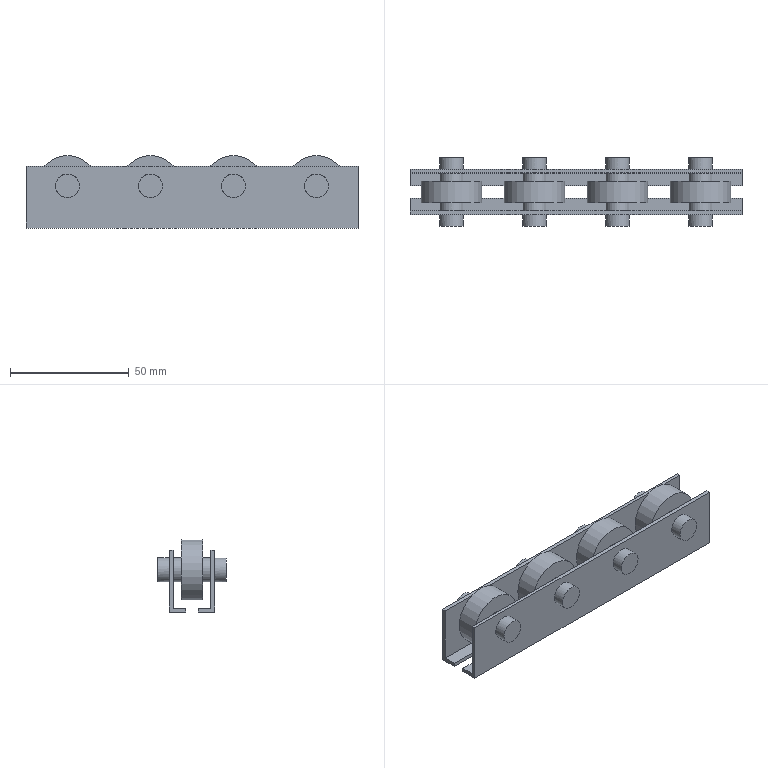Part | NX | features solid 2 | 1 solid | 52 faces | box 140 x 29 x 30.5 mm | volume 37587 mm3 | plane 32 | cylinder 20 | commonest cylinder face diameters 10 x16 25.4 x4
STEP:
#1=CARTESIAN_POINT('',(-1407.5,158.,-11.7));
#2=VERTEX_POINT('',#1);
#3=CARTESIAN_POINT('',(-1407.5,158.,-16.7));
#4=DIRECTION('',(0.,1.,0.));
#5=DIRECTION('',(0.,0.,1.));
#6=AXIS2_PLACEMENT_3D('',#3,#4,#5);
#7=CIRCLE('',#6,5.);
#8=EDGE_CURVE('',#2,#2,#7,.F.);
#9=ORIENTED_EDGE('',*,*,#8,.F.);
#10=EDGE_LOOP('',(#9));
#11=FACE_BOUND('',#10,.T.);
#12=CARTESIAN_POINT('',(-1442.5,158.,-11.7));
#13=VERTEX_POINT('',#12);
#14=CARTESIAN_POINT('',(-1442.5,158.,-16.7));
#15=DIRECTION('',(0.,1.,0.));
#16=DIRECTION('',(0.,0.,1.));
#17=AXIS2_PLACEMENT_3D('',#14,#15,#16);
#18=CIRCLE('',#17,5.);
#19=EDGE_CURVE('',#13,#13,#18,.F.);
#20=ORIENTED_EDGE('',*,*,#19,.F.);
#21=EDGE_LOOP('',(#20));
#22=FACE_BOUND('',#21,.T.);
#23=CARTESIAN_POINT('',(-1477.5,158.,-11.7));
#24=VERTEX_POINT('',#23);
#25=CARTESIAN_POINT('',(-1477.5,158.,-16.7));
#26=DIRECTION('',(0.,1.,0.));
#27=DIRECTION('',(0.,0.,1.));
#28=AXIS2_PLACEMENT_3D('',#25,#26,#27);
#29=CIRCLE('',#28,5.);
#30=EDGE_CURVE('',#24,#24,#29,.F.);
#31=ORIENTED_EDGE('',*,*,#30,.F.);
#32=EDGE_LOOP('',(#31));
#33=FACE_BOUND('',#32,.T.);
#34=CARTESIAN_POINT('',(-1512.5,158.,-11.7));
#35=VERTEX_POINT('',#34);
#36=CARTESIAN_POINT('',(-1512.5,158.,-16.7));
#37=DIRECTION('',(0.,1.,0.));
#38=DIRECTION('',(0.,0.,1.));
#39=AXIS2_PLACEMENT_3D('',#36,#37,#38);
#40=CIRCLE('',#39,5.);
#41=EDGE_CURVE('',#35,#35,#40,.F.);
#42=ORIENTED_EDGE('',*,*,#41,.F.);
#43=EDGE_LOOP('',(#42));
#44=FACE_BOUND('',#43,.T.);
#45=CARTESIAN_POINT('',(-1530.,158.,-32.9));
#46=VERTEX_POINT('',#45);
#47=CARTESIAN_POINT('',(-1390.,158.,-32.9));
#48=VERTEX_POINT('',#47);
#49=CARTESIAN_POINT('',(-3210.,158.,-32.9));
#50=DIRECTION('',(1.,0.,0.));
#51=VECTOR('',#50,1000.);
#52=LINE('',#49,#51);
#53=EDGE_CURVE('',#46,#48,#52,.T.);
#54=ORIENTED_EDGE('',*,*,#53,.T.);
#55=CARTESIAN_POINT('',(-1390.,158.,-8.5));
#56=VERTEX_POINT('',#55);
#57=CARTESIAN_POINT('',(-1390.,158.,-34.5));
#58=DIRECTION('',(0.,0.,1.));
#59=VECTOR('',#58,1000.);
#60=LINE('',#57,#59);
#61=EDGE_CURVE('',#48,#56,#60,.T.);
#62=ORIENTED_EDGE('',*,*,#61,.T.);
#63=CARTESIAN_POINT('',(-1530.,158.,-8.5));
#64=VERTEX_POINT('',#63);
#65=CARTESIAN_POINT('',(-3210.,158.,-8.5));
#66=DIRECTION('',(1.,0.,0.));
#67=VECTOR('',#66,1000.);
#68=LINE('',#65,#67);
#69=EDGE_CURVE('',#64,#56,#68,.T.);
#70=ORIENTED_EDGE('',*,*,#69,.F.);
#71=CARTESIAN_POINT('',(-1530.,158.,-34.5));
#72=DIRECTION('',(0.,0.,1.));
#73=VECTOR('',#72,1000.);
#74=LINE('',#71,#73);
#75=EDGE_CURVE('',#46,#64,#74,.T.);
#76=ORIENTED_EDGE('',*,*,#75,.F.);
#77=EDGE_LOOP('',(#54,#62,#70,#76));
#78=FACE_BOUND('',#77,.T.);
#79=CARTESIAN_POINT('',(-3210.,158.,-34.5));
#80=DIRECTION('',(0.,-1.,0.));
#81=DIRECTION('',(0.,0.,1.));
#82=AXIS2_PLACEMENT_3D('',#79,#80,#81);
#83=PLANE('',#82);
#84=ADVANCED_FACE('',(#11,#22,#33,#44,#78),#83,.T.);
#85=CARTESIAN_POINT('',(-1407.5,159.6,-11.7));
#86=VERTEX_POINT('',#85);
#87=CARTESIAN_POINT('',(-1407.5,159.6,-16.7));
#88=DIRECTION('',(0.,1.,0.));
#89=DIRECTION('',(0.,0.,1.));
#90=AXIS2_PLACEMENT_3D('',#87,#88,#89);
#91=CIRCLE('',#90,5.);
#92=EDGE_CURVE('',#86,#86,#91,.F.);
#93=ORIENTED_EDGE('',*,*,#92,.T.);
#94=EDGE_LOOP('',(#93));
#95=FACE_BOUND('',#94,.T.);
#96=CARTESIAN_POINT('',(-1442.5,159.6,-11.7));
#97=VERTEX_POINT('',#96);
#98=CARTESIAN_POINT('',(-1442.5,159.6,-16.7));
#99=DIRECTION('',(0.,1.,0.));
#100=DIRECTION('',(0.,0.,1.));
#101=AXIS2_PLACEMENT_3D('',#98,#99,#100);
#102=CIRCLE('',#101,5.);
#103=EDGE_CURVE('',#97,#97,#102,.F.);
#104=ORIENTED_EDGE('',*,*,#103,.T.);
#105=EDGE_LOOP('',(#104));
#106=FACE_BOUND('',#105,.T.);
#107=CARTESIAN_POINT('',(-1477.5,159.6,-11.7));
#108=VERTEX_POINT('',#107);
#109=CARTESIAN_POINT('',(-1477.5,159.6,-16.7));
#110=DIRECTION('',(0.,1.,0.));
#111=DIRECTION('',(0.,0.,1.));
#112=AXIS2_PLACEMENT_3D('',#109,#110,#111);
#113=CIRCLE('',#112,5.);
#114=EDGE_CURVE('',#108,#108,#113,.F.);
#115=ORIENTED_EDGE('',*,*,#114,.T.);
#116=EDGE_LOOP('',(#115));
#117=FACE_BOUND('',#116,.T.);
#118=CARTESIAN_POINT('',(-1512.5,159.6,-11.7));
#119=VERTEX_POINT('',#118);
#120=CARTESIAN_POINT('',(-1512.5,159.6,-16.7));
#121=DIRECTION('',(0.,1.,0.));
#122=DIRECTION('',(0.,0.,1.));
#123=AXIS2_PLACEMENT_3D('',#120,#121,#122);
#124=CIRCLE('',#123,5.);
#125=EDGE_CURVE('',#119,#119,#124,.F.);
#126=ORIENTED_EDGE('',*,*,#125,.T.);
#127=EDGE_LOOP('',(#126));
#128=FACE_BOUND('',#127,.T.);
#129=CARTESIAN_POINT('',(-1390.,159.6,-34.5));
#130=VERTEX_POINT('',#129);
#131=CARTESIAN_POINT('',(-1390.,159.6,-8.5));
#132=VERTEX_POINT('',#131);
#133=CARTESIAN_POINT('',(-1390.,159.6,-34.5));
#134=DIRECTION('',(0.,0.,1.));
#135=VECTOR('',#134,1000.);
#136=LINE('',#133,#135);
#137=EDGE_CURVE('',#130,#132,#136,.T.);
#138=ORIENTED_EDGE('',*,*,#137,.F.);
#139=CARTESIAN_POINT('',(-1530.,159.6,-34.5));
#140=VERTEX_POINT('',#139);
#141=CARTESIAN_POINT('',(-2230.,159.6,-34.5));
#142=DIRECTION('',(-1.,0.,0.));
#143=VECTOR('',#142,1000.);
#144=LINE('',#141,#143);
#145=EDGE_CURVE('',#130,#140,#144,.T.);
#146=ORIENTED_EDGE('',*,*,#145,.T.);
#147=CARTESIAN_POINT('',(-1530.,159.6,-8.5));
#148=VERTEX_POINT('',#147);
#149=CARTESIAN_POINT('',(-1530.,159.6,-34.5));
#150=DIRECTION('',(0.,0.,1.));
#151=VECTOR('',#150,1000.);
#152=LINE('',#149,#151);
#153=EDGE_CURVE('',#140,#148,#152,.T.);
#154=ORIENTED_EDGE('',*,*,#153,.T.);
#155=CARTESIAN_POINT('',(-3210.,159.6,-8.5));
#156=DIRECTION('',(1.,0.,0.));
#157=VECTOR('',#156,1000.);
#158=LINE('',#155,#157);
#159=EDGE_CURVE('',#148,#132,#158,.T.);
#160=ORIENTED_EDGE('',*,*,#159,.T.);
#161=EDGE_LOOP('',(#138,#146,#154,#160));
#162=FACE_BOUND('',#161,.T.);
#163=CARTESIAN_POINT('',(-3210.,159.6,-34.5));
#164=DIRECTION('',(0.,-1.,0.));
#165=DIRECTION('',(0.,0.,1.));
#166=AXIS2_PLACEMENT_3D('',#163,#164,#165);
#167=PLANE('',#166);
#168=ADVANCED_FACE('',(#95,#106,#117,#128,#162),#167,.F.);
#169=ORIENTED_EDGE('',*,*,#145,.F.);
#170=CARTESIAN_POINT('',(-1390.,152.6,-34.5));
#171=VERTEX_POINT('',#170);
#172=CARTESIAN_POINT('',(-1390.,159.6,-34.5));
#173=DIRECTION('',(0.,-1.,0.));
#174=VECTOR('',#173,1000.);
#175=LINE('',#172,#174);
#176=EDGE_CURVE('',#130,#171,#175,.T.);
#177=ORIENTED_EDGE('',*,*,#176,.T.);
#178=CARTESIAN_POINT('',(-1530.,152.6,-34.5));
#179=VERTEX_POINT('',#178);
#180=CARTESIAN_POINT('',(-2230.,152.6,-34.5));
#181=DIRECTION('',(-1.,0.,0.));
#182=VECTOR('',#181,1000.);
#183=LINE('',#180,#182);
#184=EDGE_CURVE('',#171,#179,#183,.T.);
#185=ORIENTED_EDGE('',*,*,#184,.T.);
#186=CARTESIAN_POINT('',(-1530.,159.6,-34.5));
#187=DIRECTION('',(0.,-1.,0.));
#188=VECTOR('',#187,1000.);
#189=LINE('',#186,#188);
#190=EDGE_CURVE('',#140,#179,#189,.T.);
#191=ORIENTED_EDGE('',*,*,#190,.F.);
#192=EDGE_LOOP('',(#169,#177,#185,#191));
#193=FACE_BOUND('',#192,.T.);
#194=CARTESIAN_POINT('',(-2230.,159.6,-34.5));
#195=DIRECTION('',(0.,0.,-1.));
#196=DIRECTION('',(1.,0.,0.));
#197=AXIS2_PLACEMENT_3D('',#194,#195,#196);
#198=PLANE('',#197);
#199=ADVANCED_FACE('',(#193),#198,.T.);
#200=CARTESIAN_POINT('',(-1390.,152.6,-32.9));
#201=VERTEX_POINT('',#200);
#202=CARTESIAN_POINT('',(-1390.,152.6,-34.5));
#203=DIRECTION('',(0.,0.,1.));
#204=VECTOR('',#203,1000.);
#205=LINE('',#202,#204);
#206=EDGE_CURVE('',#201,#171,#205,.F.);
#207=ORIENTED_EDGE('',*,*,#206,.F.);
#208=CARTESIAN_POINT('',(-1530.,152.6,-32.9));
#209=VERTEX_POINT('',#208);
#210=CARTESIAN_POINT('',(-2230.,152.6,-32.9));
#211=DIRECTION('',(-1.,0.,0.));
#212=VECTOR('',#211,1000.);
#213=LINE('',#210,#212);
#214=EDGE_CURVE('',#201,#209,#213,.T.);
#215=ORIENTED_EDGE('',*,*,#214,.T.);
#216=CARTESIAN_POINT('',(-1530.,152.6,-34.5));
#217=DIRECTION('',(0.,0.,1.));
#218=VECTOR('',#217,1000.);
#219=LINE('',#216,#218);
#220=EDGE_CURVE('',#209,#179,#219,.F.);
#221=ORIENTED_EDGE('',*,*,#220,.T.);
#222=ORIENTED_EDGE('',*,*,#184,.F.);
#223=EDGE_LOOP('',(#207,#215,#221,#222));
#224=FACE_BOUND('',#223,.T.);
#225=CARTESIAN_POINT('',(-2230.,152.6,-34.5));
#226=DIRECTION('',(0.,-1.,0.));
#227=DIRECTION('',(-1.,0.,0.));
#228=AXIS2_PLACEMENT_3D('',#225,#226,#227);
#229=PLANE('',#228);
#230=ADVANCED_FACE('',(#224),#229,.T.);
#231=ORIENTED_EDGE('',*,*,#214,.F.);
#232=CARTESIAN_POINT('',(-1390.,152.6,-32.9));
#233=DIRECTION('',(0.,1.,0.));
#234=VECTOR('',#233,1000.);
#235=LINE('',#232,#234);
#236=EDGE_CURVE('',#201,#48,#235,.T.);
#237=ORIENTED_EDGE('',*,*,#236,.T.);
#238=ORIENTED_EDGE('',*,*,#53,.F.);
#239=CARTESIAN_POINT('',(-1530.,152.6,-32.9));
#240=DIRECTION('',(0.,1.,0.));
#241=VECTOR('',#240,1000.);
#242=LINE('',#239,#241);
#243=EDGE_CURVE('',#209,#46,#242,.T.);
#244=ORIENTED_EDGE('',*,*,#243,.F.);
#245=EDGE_LOOP('',(#231,#237,#238,#244));
#246=FACE_BOUND('',#245,.T.);
#247=CARTESIAN_POINT('',(-2230.,152.6,-32.9));
#248=DIRECTION('',(0.,0.,1.));
#249=DIRECTION('',(-1.,0.,0.));
#250=AXIS2_PLACEMENT_3D('',#247,#248,#249);
#251=PLANE('',#250);
#252=ADVANCED_FACE('',(#246),#251,.T.);
#253=ORIENTED_EDGE('',*,*,#69,.T.);
#254=CARTESIAN_POINT('',(-1390.,159.6,-8.5));
#255=DIRECTION('',(0.,1.,0.));
#256=VECTOR('',#255,1000.);
#257=LINE('',#254,#256);
#258=EDGE_CURVE('',#56,#132,#257,.T.);
#259=ORIENTED_EDGE('',*,*,#258,.T.);
#260=ORIENTED_EDGE('',*,*,#159,.F.);
#261=CARTESIAN_POINT('',(-1530.,159.6,-8.5));
#262=DIRECTION('',(0.,1.,0.));
#263=VECTOR('',#262,1000.);
#264=LINE('',#261,#263);
#265=EDGE_CURVE('',#64,#148,#264,.T.);
#266=ORIENTED_EDGE('',*,*,#265,.F.);
#267=EDGE_LOOP('',(#253,#259,#260,#266));
#268=FACE_BOUND('',#267,.T.);
#269=CARTESIAN_POINT('',(-3210.,159.6,-8.5));
#270=DIRECTION('',(0.,0.,1.));
#271=DIRECTION('',(0.,1.,0.));
#272=AXIS2_PLACEMENT_3D('',#269,#270,#271);
#273=PLANE('',#272);
#274=ADVANCED_FACE('',(#268),#273,.T.);
#275=CARTESIAN_POINT('',(-1407.5,140.4,-21.7));
#276=VERTEX_POINT('',#275);
#277=CARTESIAN_POINT('',(-1407.5,140.4,-16.7));
#278=DIRECTION('',(0.,-1.,0.));
#279=DIRECTION('',(0.,0.,-1.));
#280=AXIS2_PLACEMENT_3D('',#277,#278,#279);
#281=CIRCLE('',#280,5.);
#282=EDGE_CURVE('',#276,#276,#281,.T.);
#283=ORIENTED_EDGE('',*,*,#282,.F.);
#284=EDGE_LOOP('',(#283));
#285=FACE_BOUND('',#284,.T.);
#286=CARTESIAN_POINT('',(-1442.5,140.4,-21.7));
#287=VERTEX_POINT('',#286);
#288=CARTESIAN_POINT('',(-1442.5,140.4,-16.7));
#289=DIRECTION('',(0.,-1.,0.));
#290=DIRECTION('',(0.,0.,-1.));
#291=AXIS2_PLACEMENT_3D('',#288,#289,#290);
#292=CIRCLE('',#291,5.);
#293=EDGE_CURVE('',#287,#287,#292,.T.);
#294=ORIENTED_EDGE('',*,*,#293,.F.);
#295=EDGE_LOOP('',(#294));
#296=FACE_BOUND('',#295,.T.);
#297=CARTESIAN_POINT('',(-1477.5,140.4,-21.7));
#298=VERTEX_POINT('',#297);
#299=CARTESIAN_POINT('',(-1477.5,140.4,-16.7));
#300=DIRECTION('',(0.,-1.,0.));
#301=DIRECTION('',(0.,0.,-1.));
#302=AXIS2_PLACEMENT_3D('',#299,#300,#301);
#303=CIRCLE('',#302,5.);
#304=EDGE_CURVE('',#298,#298,#303,.T.);
#305=ORIENTED_EDGE('',*,*,#304,.F.);
#306=EDGE_LOOP('',(#305));
#307=FACE_BOUND('',#306,.T.);
#308=CARTESIAN_POINT('',(-1512.5,140.4,-21.7));
#309=VERTEX_POINT('',#308);
#310=CARTESIAN_POINT('',(-1512.5,140.4,-16.7));
#311=DIRECTION('',(0.,-1.,0.));
#312=DIRECTION('',(0.,0.,-1.));
#313=AXIS2_PLACEMENT_3D('',#310,#311,#312);
#314=CIRCLE('',#313,5.);
#315=EDGE_CURVE('',#309,#309,#314,.T.);
#316=ORIENTED_EDGE('',*,*,#315,.F.);
#317=EDGE_LOOP('',(#316));
#318=FACE_BOUND('',#317,.T.);
#319=CARTESIAN_POINT('',(-1390.,140.4,-8.5));
#320=VERTEX_POINT('',#319);
#321=CARTESIAN_POINT('',(-1390.,140.4,-34.5));
#322=VERTEX_POINT('',#321);
#323=CARTESIAN_POINT('',(-1390.,140.4,-34.5));
#324=DIRECTION('',(0.,0.,-1.));
#325=VECTOR('',#324,1000.);
#326=LINE('',#323,#325);
#327=EDGE_CURVE('',#320,#322,#326,.T.);
#328=ORIENTED_EDGE('',*,*,#327,.F.);
#329=CARTESIAN_POINT('',(-1530.,140.4,-8.5));
#330=VERTEX_POINT('',#329);
#331=CARTESIAN_POINT('',(-3210.,140.4,-8.5));
#332=DIRECTION('',(1.,0.,0.));
#333=VECTOR('',#332,1000.);
#334=LINE('',#331,#333);
#335=EDGE_CURVE('',#330,#320,#334,.T.);
#336=ORIENTED_EDGE('',*,*,#335,.F.);
#337=CARTESIAN_POINT('',(-1530.,140.4,-34.5));
#338=VERTEX_POINT('',#337);
#339=CARTESIAN_POINT('',(-1530.,140.4,-34.5));
#340=DIRECTION('',(0.,0.,-1.));
#341=VECTOR('',#340,1000.);
#342=LINE('',#339,#341);
#343=EDGE_CURVE('',#330,#338,#342,.T.);
#344=ORIENTED_EDGE('',*,*,#343,.T.);
#345=CARTESIAN_POINT('',(-2230.,140.4,-34.5));
#346=DIRECTION('',(-1.,0.,0.));
#347=VECTOR('',#346,1000.);
#348=LINE('',#345,#347);
#349=EDGE_CURVE('',#322,#338,#348,.T.);
#350=ORIENTED_EDGE('',*,*,#349,.F.);
#351=EDGE_LOOP('',(#328,#336,#344,#350));
#352=FACE_BOUND('',#351,.T.);
#353=CARTESIAN_POINT('',(-2230.,140.4,-34.5));
#354=DIRECTION('',(0.,1.,0.));
#355=DIRECTION('',(-1.,0.,0.));
#356=AXIS2_PLACEMENT_3D('',#353,#354,#355);
#357=PLANE('',#356);
#358=ADVANCED_FACE('',(#285,#296,#307,#318,#352),#357,.F.);
#359=CARTESIAN_POINT('',(-1407.5,142.,-11.7));
#360=VERTEX_POINT('',#359);
#361=CARTESIAN_POINT('',(-1407.5,142.,-16.7));
#362=DIRECTION('',(0.,1.,0.));
#363=DIRECTION('',(0.,0.,1.));
#364=AXIS2_PLACEMENT_3D('',#361,#362,#363);
#365=CIRCLE('',#364,5.);
#366=EDGE_CURVE('',#360,#360,#365,.T.);
#367=ORIENTED_EDGE('',*,*,#366,.F.);
#368=EDGE_LOOP('',(#367));
#369=FACE_BOUND('',#368,.T.);
#370=CARTESIAN_POINT('',(-1442.5,142.,-11.7));
#371=VERTEX_POINT('',#370);
#372=CARTESIAN_POINT('',(-1442.5,142.,-16.7));
#373=DIRECTION('',(0.,1.,0.));
#374=DIRECTION('',(0.,0.,1.));
#375=AXIS2_PLACEMENT_3D('',#372,#373,#374);
#376=CIRCLE('',#375,5.);
#377=EDGE_CURVE('',#371,#371,#376,.T.);
#378=ORIENTED_EDGE('',*,*,#377,.F.);
#379=EDGE_LOOP('',(#378));
#380=FACE_BOUND('',#379,.T.);
#381=CARTESIAN_POINT('',(-1477.5,142.,-11.7));
#382=VERTEX_POINT('',#381);
#383=CARTESIAN_POINT('',(-1477.5,142.,-16.7));
#384=DIRECTION('',(0.,1.,0.));
#385=DIRECTION('',(0.,0.,1.));
#386=AXIS2_PLACEMENT_3D('',#383,#384,#385);
#387=CIRCLE('',#386,5.);
#388=EDGE_CURVE('',#382,#382,#387,.T.);
#389=ORIENTED_EDGE('',*,*,#388,.F.);
#390=EDGE_LOOP('',(#389));
#391=FACE_BOUND('',#390,.T.);
#392=CARTESIAN_POINT('',(-1512.5,142.,-11.7));
#393=VERTEX_POINT('',#392);
#394=CARTESIAN_POINT('',(-1512.5,142.,-16.7));
#395=DIRECTION('',(0.,1.,0.));
#396=DIRECTION('',(0.,0.,1.));
#397=AXIS2_PLACEMENT_3D('',#394,#395,#396);
#398=CIRCLE('',#397,5.);
#399=EDGE_CURVE('',#393,#393,#398,.T.);
#400=ORIENTED_EDGE('',*,*,#399,.F.);
#401=EDGE_LOOP('',(#400));
#402=FACE_BOUND('',#401,.T.);
#403=CARTESIAN_POINT('',(-1390.,142.,-32.9));
#404=VERTEX_POINT('',#403);
#405=CARTESIAN_POINT('',(-1390.,142.,-8.5));
#406=VERTEX_POINT('',#405);
#407=CARTESIAN_POINT('',(-1390.,142.,-34.5));
#408=DIRECTION('',(0.,0.,1.));
#409=VECTOR('',#408,1000.);
#410=LINE('',#407,#409);
#411=EDGE_CURVE('',#404,#406,#410,.T.);
#412=ORIENTED_EDGE('',*,*,#411,.F.);
#413=CARTESIAN_POINT('',(-1530.,142.,-32.9));
#414=VERTEX_POINT('',#413);
#415=CARTESIAN_POINT('',(-2230.,142.,-32.9));
#416=DIRECTION('',(1.,0.,0.));
#417=VECTOR('',#416,1000.);
#418=LINE('',#415,#417);
#419=EDGE_CURVE('',#414,#404,#418,.T.);
#420=ORIENTED_EDGE('',*,*,#419,.F.);
#421=CARTESIAN_POINT('',(-1530.,142.,-8.5));
#422=VERTEX_POINT('',#421);
#423=CARTESIAN_POINT('',(-1530.,142.,-34.5));
#424=DIRECTION('',(0.,0.,1.));
#425=VECTOR('',#424,1000.);
#426=LINE('',#423,#425);
#427=EDGE_CURVE('',#414,#422,#426,.T.);
#428=ORIENTED_EDGE('',*,*,#427,.T.);
#429=CARTESIAN_POINT('',(-3210.,142.,-8.5));
#430=DIRECTION('',(1.,0.,0.));
#431=VECTOR('',#430,1000.);
#432=LINE('',#429,#431);
#433=EDGE_CURVE('',#422,#406,#432,.T.);
#434=ORIENTED_EDGE('',*,*,#433,.T.);
#435=EDGE_LOOP('',(#412,#420,#428,#434));
#436=FACE_BOUND('',#435,.T.);
#437=CARTESIAN_POINT('',(-3210.,142.,-34.5));
#438=DIRECTION('',(0.,-1.,0.));
#439=DIRECTION('',(0.,0.,1.));
#440=AXIS2_PLACEMENT_3D('',#437,#438,#439);
#441=PLANE('',#440);
#442=ADVANCED_FACE('',(#369,#380,#391,#402,#436),#441,.F.);
#443=CARTESIAN_POINT('',(-1390.,140.4,-8.5));
#444=DIRECTION('',(0.,-1.,0.));
#445=VECTOR('',#444,1000.);
#446=LINE('',#443,#445);
#447=EDGE_CURVE('',#406,#320,#446,.T.);
#448=ORIENTED_EDGE('',*,*,#447,.F.);
#449=ORIENTED_EDGE('',*,*,#433,.F.);
#450=CARTESIAN_POINT('',(-1530.,140.4,-8.5));
#451=DIRECTION('',(0.,-1.,0.));
#452=VECTOR('',#451,1000.);
#453=LINE('',#450,#452);
#454=EDGE_CURVE('',#422,#330,#453,.T.);
#455=ORIENTED_EDGE('',*,*,#454,.T.);
#456=ORIENTED_EDGE('',*,*,#335,.T.);
#457=EDGE_LOOP('',(#448,#449,#455,#456));
#458=FACE_BOUND('',#457,.T.);
#459=CARTESIAN_POINT('',(-3210.,140.4,-8.5));
#460=DIRECTION('',(0.,0.,-1.));
#461=DIRECTION('',(0.,-1.,0.));
#462=AXIS2_PLACEMENT_3D('',#459,#460,#461);
#463=PLANE('',#462);
#464=ADVANCED_FACE('',(#458),#463,.F.);
#465=CARTESIAN_POINT('',(-1390.,147.4,-32.9));
#466=VERTEX_POINT('',#465);
#467=CARTESIAN_POINT('',(-1390.,147.4,-32.9));
#468=DIRECTION('',(0.,-1.,0.));
#469=VECTOR('',#468,1000.);
#470=LINE('',#467,#469);
#471=EDGE_CURVE('',#466,#404,#470,.T.);
#472=ORIENTED_EDGE('',*,*,#471,.F.);
#473=CARTESIAN_POINT('',(-1530.,147.4,-32.9));
#474=VERTEX_POINT('',#473);
#475=CARTESIAN_POINT('',(-2230.,147.4,-32.9));
#476=DIRECTION('',(1.,0.,0.));
#477=VECTOR('',#476,1000.);
#478=LINE('',#475,#477);
#479=EDGE_CURVE('',#466,#474,#478,.F.);
#480=ORIENTED_EDGE('',*,*,#479,.T.);
#481=CARTESIAN_POINT('',(-1530.,147.4,-32.9));
#482=DIRECTION('',(0.,-1.,0.));
#483=VECTOR('',#482,1000.);
#484=LINE('',#481,#483);
#485=EDGE_CURVE('',#474,#414,#484,.T.);
#486=ORIENTED_EDGE('',*,*,#485,.T.);
#487=ORIENTED_EDGE('',*,*,#419,.T.);
#488=EDGE_LOOP('',(#472,#480,#486,#487));
#489=FACE_BOUND('',#488,.T.);
#490=CARTESIAN_POINT('',(-2230.,147.4,-32.9));
#491=DIRECTION('',(0.,0.,-1.));
#492=DIRECTION('',(1.,0.,0.));
#493=AXIS2_PLACEMENT_3D('',#490,#491,#492);
#494=PLANE('',#493);
#495=ADVANCED_FACE('',(#489),#494,.F.);
#496=CARTESIAN_POINT('',(-1390.,147.4,-34.5));
#497=VERTEX_POINT('',#496);
#498=CARTESIAN_POINT('',(-1390.,147.4,-34.5));
#499=DIRECTION('',(0.,0.,-1.));
#500=VECTOR('',#499,1000.);
#501=LINE('',#498,#500);
#502=EDGE_CURVE('',#497,#466,#501,.F.);
#503=ORIENTED_EDGE('',*,*,#502,.F.);
#504=CARTESIAN_POINT('',(-1530.,147.4,-34.5));
#505=VERTEX_POINT('',#504);
#506=CARTESIAN_POINT('',(-2230.,147.4,-34.5));
#507=DIRECTION('',(-1.,0.,0.));
#508=VECTOR('',#507,1000.);
#509=LINE('',#506,#508);
#510=EDGE_CURVE('',#497,#505,#509,.T.);
#511=ORIENTED_EDGE('',*,*,#510,.T.);
#512=CARTESIAN_POINT('',(-1530.,147.4,-34.5));
#513=DIRECTION('',(0.,0.,-1.));
#514=VECTOR('',#513,1000.);
#515=LINE('',#512,#514);
#516=EDGE_CURVE('',#505,#474,#515,.F.);
#517=ORIENTED_EDGE('',*,*,#516,.T.);
#518=ORIENTED_EDGE('',*,*,#479,.F.);
#519=EDGE_LOOP('',(#503,#511,#517,#518));
#520=FACE_BOUND('',#519,.T.);
#521=CARTESIAN_POINT('',(-2230.,147.4,-34.5));
#522=DIRECTION('',(0.,1.,0.));
#523=DIRECTION('',(-1.,0.,0.));
#524=AXIS2_PLACEMENT_3D('',#521,#522,#523);
#525=PLANE('',#524);
#526=ADVANCED_FACE('',(#520),#525,.T.);
#527=ORIENTED_EDGE('',*,*,#510,.F.);
#528=CARTESIAN_POINT('',(-1390.,147.4,-34.5));
#529=DIRECTION('',(0.,-1.,0.));
#530=VECTOR('',#529,1000.);
#531=LINE('',#528,#530);
#532=EDGE_CURVE('',#497,#322,#531,.T.);
#533=ORIENTED_EDGE('',*,*,#532,.T.);
#534=ORIENTED_EDGE('',*,*,#349,.T.);
#535=CARTESIAN_POINT('',(-1530.,147.4,-34.5));
#536=DIRECTION('',(0.,-1.,0.));
#537=VECTOR('',#536,1000.);
#538=LINE('',#535,#537);
#539=EDGE_CURVE('',#505,#338,#538,.T.);
#540=ORIENTED_EDGE('',*,*,#539,.F.);
#541=EDGE_LOOP('',(#527,#533,#534,#540));
#542=FACE_BOUND('',#541,.T.);
#543=CARTESIAN_POINT('',(-2230.,147.4,-34.5));
#544=DIRECTION('',(0.,0.,-1.));
#545=DIRECTION('',(1.,0.,0.));
#546=AXIS2_PLACEMENT_3D('',#543,#544,#545);
#547=PLANE('',#546);
#548=ADVANCED_FACE('',(#542),#547,.T.);
#549=CARTESIAN_POINT('',(-1499.8,154.5,-16.7));
#550=VERTEX_POINT('',#549);
#551=CARTESIAN_POINT('',(-1512.5,154.5,-16.7));
#552=DIRECTION('',(0.,-1.,0.));
#553=DIRECTION('',(1.,0.,0.));
#554=AXIS2_PLACEMENT_3D('',#551,#552,#553);
#555=CIRCLE('',#554,12.7);
#556=EDGE_CURVE('',#550,#550,#555,.T.);
#557=ORIENTED_EDGE('',*,*,#556,.T.);
#558=EDGE_LOOP('',(#557));
#559=FACE_BOUND('',#558,.T.);
#560=CARTESIAN_POINT('',(-1499.8,145.5,-16.7));
#561=VERTEX_POINT('',#560);
#562=CARTESIAN_POINT('',(-1512.5,145.5,-16.7));
#563=DIRECTION('',(0.,-1.,0.));
#564=DIRECTION('',(1.,0.,0.));
#565=AXIS2_PLACEMENT_3D('',#562,#563,#564);
#566=CIRCLE('',#565,12.7);
#567=EDGE_CURVE('',#561,#561,#566,.T.);
#568=ORIENTED_EDGE('',*,*,#567,.F.);
#569=EDGE_LOOP('',(#568));
#570=FACE_BOUND('',#569,.T.);
#571=CARTESIAN_POINT('',(-1512.5,154.5,-16.7));
#572=DIRECTION('',(0.,-1.,0.));
#573=DIRECTION('',(0.,0.,1.));
#574=AXIS2_PLACEMENT_3D('',#571,#572,#573);
#575=CYLINDRICAL_SURFACE('',#574,12.7);
#576=ADVANCED_FACE('',(#559,#570),#575,.T.);
#577=CARTESIAN_POINT('',(-1464.8,154.5,-16.7));
#578=VERTEX_POINT('',#577);
#579=CARTESIAN_POINT('',(-1477.5,154.5,-16.7));
#580=DIRECTION('',(0.,-1.,0.));
#581=DIRECTION('',(1.,0.,0.));
#582=AXIS2_PLACEMENT_3D('',#579,#580,#581);
#583=CIRCLE('',#582,12.7);
#584=EDGE_CURVE('',#578,#578,#583,.T.);
#585=ORIENTED_EDGE('',*,*,#584,.T.);
#586=EDGE_LOOP('',(#585));
#587=FACE_BOUND('',#586,.T.);
#588=CARTESIAN_POINT('',(-1464.8,145.5,-16.7));
#589=VERTEX_POINT('',#588);
#590=CARTESIAN_POINT('',(-1477.5,145.5,-16.7));
#591=DIRECTION('',(0.,-1.,0.));
#592=DIRECTION('',(1.,0.,0.));
#593=AXIS2_PLACEMENT_3D('',#590,#591,#592);
#594=CIRCLE('',#593,12.7);
#595=EDGE_CURVE('',#589,#589,#594,.T.);
#596=ORIENTED_EDGE('',*,*,#595,.F.);
#597=EDGE_LOOP('',(#596));
#598=FACE_BOUND('',#597,.T.);
#599=CARTESIAN_POINT('',(-1477.5,154.5,-16.7));
#600=DIRECTION('',(0.,-1.,0.));
#601=DIRECTION('',(0.,0.,1.));
#602=AXIS2_PLACEMENT_3D('',#599,#600,#601);
#603=CYLINDRICAL_SURFACE('',#602,12.7);
#604=ADVANCED_FACE('',(#587,#598),#603,.T.);
#605=CARTESIAN_POINT('',(-1429.8,154.5,-16.7));
#606=VERTEX_POINT('',#605);
#607=CARTESIAN_POINT('',(-1442.5,154.5,-16.7));
#608=DIRECTION('',(0.,-1.,0.));
#609=DIRECTION('',(1.,0.,0.));
#610=AXIS2_PLACEMENT_3D('',#607,#608,#609);
#611=CIRCLE('',#610,12.7);
#612=EDGE_CURVE('',#606,#606,#611,.T.);
#613=ORIENTED_EDGE('',*,*,#612,.T.);
#614=EDGE_LOOP('',(#613));
#615=FACE_BOUND('',#614,.T.);
#616=CARTESIAN_POINT('',(-1429.8,145.5,-16.7));
#617=VERTEX_POINT('',#616);
#618=CARTESIAN_POINT('',(-1442.5,145.5,-16.7));
#619=DIRECTION('',(0.,-1.,0.));
#620=DIRECTION('',(1.,0.,0.));
#621=AXIS2_PLACEMENT_3D('',#618,#619,#620);
#622=CIRCLE('',#621,12.7);
#623=EDGE_CURVE('',#617,#617,#622,.T.);
#624=ORIENTED_EDGE('',*,*,#623,.F.);
#625=EDGE_LOOP('',(#624));
#626=FACE_BOUND('',#625,.T.);
#627=CARTESIAN_POINT('',(-1442.5,154.5,-16.7));
#628=DIRECTION('',(0.,-1.,0.));
#629=DIRECTION('',(0.,0.,1.));
#630=AXIS2_PLACEMENT_3D('',#627,#628,#629);
#631=CYLINDRICAL_SURFACE('',#630,12.7);
#632=ADVANCED_FACE('',(#615,#626),#631,.T.);
#633=CARTESIAN_POINT('',(-1394.8,154.5,-16.7));
#634=VERTEX_POINT('',#633);
#635=CARTESIAN_POINT('',(-1407.5,154.5,-16.7));
#636=DIRECTION('',(0.,-1.,0.));
#637=DIRECTION('',(1.,0.,0.));
#638=AXIS2_PLACEMENT_3D('',#635,#636,#637);
#639=CIRCLE('',#638,12.7);
#640=EDGE_CURVE('',#634,#634,#639,.T.);
#641=ORIENTED_EDGE('',*,*,#640,.T.);
#642=EDGE_LOOP('',(#641));
#643=FACE_BOUND('',#642,.T.);
#644=CARTESIAN_POINT('',(-1394.8,145.5,-16.7));
#645=VERTEX_POINT('',#644);
#646=CARTESIAN_POINT('',(-1407.5,145.5,-16.7));
#647=DIRECTION('',(0.,-1.,0.));
#648=DIRECTION('',(1.,0.,0.));
#649=AXIS2_PLACEMENT_3D('',#646,#647,#648);
#650=CIRCLE('',#649,12.7);
#651=EDGE_CURVE('',#645,#645,#650,.T.);
#652=ORIENTED_EDGE('',*,*,#651,.F.);
#653=EDGE_LOOP('',(#652));
#654=FACE_BOUND('',#653,.T.);
#655=CARTESIAN_POINT('',(-1407.5,154.5,-16.7));
#656=DIRECTION('',(0.,-1.,0.));
#657=DIRECTION('',(0.,0.,1.));
#658=AXIS2_PLACEMENT_3D('',#655,#656,#657);
#659=CYLINDRICAL_SURFACE('',#658,12.7);
#660=ADVANCED_FACE('',(#643,#654),#659,.T.);
#661=CARTESIAN_POINT('',(-1507.5,164.5,-16.7));
#662=VERTEX_POINT('',#661);
#663=CARTESIAN_POINT('',(-1512.5,164.5,-16.7));
#664=DIRECTION('',(0.,-1.,0.));
#665=DIRECTION('',(1.,0.,0.));
#666=AXIS2_PLACEMENT_3D('',#663,#664,#665);
#667=CIRCLE('',#666,5.);
#668=EDGE_CURVE('',#662,#662,#667,.T.);
#669=ORIENTED_EDGE('',*,*,#668,.F.);
#670=EDGE_LOOP('',(#669));
#671=FACE_BOUND('',#670,.T.);
#672=CARTESIAN_POINT('',(-1512.5,164.5,-16.7));
#673=DIRECTION('',(0.,1.,0.));
#674=DIRECTION('',(0.,0.,-1.));
#675=AXIS2_PLACEMENT_3D('',#672,#673,#674);
#676=PLANE('',#675);
#677=ADVANCED_FACE('',(#671),#676,.T.);
#678=CARTESIAN_POINT('',(-1472.5,164.5,-16.7));
#679=VERTEX_POINT('',#678);
#680=CARTESIAN_POINT('',(-1477.5,164.5,-16.7));
#681=DIRECTION('',(0.,-1.,0.));
#682=DIRECTION('',(1.,0.,0.));
#683=AXIS2_PLACEMENT_3D('',#680,#681,#682);
#684=CIRCLE('',#683,5.);
#685=EDGE_CURVE('',#679,#679,#684,.T.);
#686=ORIENTED_EDGE('',*,*,#685,.F.);
#687=EDGE_LOOP('',(#686));
#688=FACE_BOUND('',#687,.T.);
#689=CARTESIAN_POINT('',(-1477.5,164.5,-16.7));
#690=DIRECTION('',(0.,1.,0.));
#691=DIRECTION('',(0.,0.,-1.));
#692=AXIS2_PLACEMENT_3D('',#689,#690,#691);
#693=PLANE('',#692);
#694=ADVANCED_FACE('',(#688),#693,.T.);
#695=CARTESIAN_POINT('',(-1437.5,164.5,-16.7));
#696=VERTEX_POINT('',#695);
#697=CARTESIAN_POINT('',(-1442.5,164.5,-16.7));
#698=DIRECTION('',(0.,-1.,0.));
#699=DIRECTION('',(1.,0.,0.));
#700=AXIS2_PLACEMENT_3D('',#697,#698,#699);
#701=CIRCLE('',#700,5.);
#702=EDGE_CURVE('',#696,#696,#701,.T.);
#703=ORIENTED_EDGE('',*,*,#702,.F.);
#704=EDGE_LOOP('',(#703));
#705=FACE_BOUND('',#704,.T.);
#706=CARTESIAN_POINT('',(-1442.5,164.5,-16.7));
#707=DIRECTION('',(0.,1.,0.));
#708=DIRECTION('',(0.,0.,-1.));
#709=AXIS2_PLACEMENT_3D('',#706,#707,#708);
#710=PLANE('',#709);
#711=ADVANCED_FACE('',(#705),#710,.T.);
#712=CARTESIAN_POINT('',(-1402.5,164.5,-16.7));
#713=VERTEX_POINT('',#712);
#714=CARTESIAN_POINT('',(-1407.5,164.5,-16.7));
#715=DIRECTION('',(0.,-1.,0.));
#716=DIRECTION('',(1.,0.,0.));
#717=AXIS2_PLACEMENT_3D('',#714,#715,#716);
#718=CIRCLE('',#717,5.);
#719=EDGE_CURVE('',#713,#713,#718,.T.);
#720=ORIENTED_EDGE('',*,*,#719,.F.);
#721=EDGE_LOOP('',(#720));
#722=FACE_BOUND('',#721,.T.);
#723=CARTESIAN_POINT('',(-1407.5,164.5,-16.7));
#724=DIRECTION('',(0.,1.,0.));
#725=DIRECTION('',(0.,0.,-1.));
#726=AXIS2_PLACEMENT_3D('',#723,#724,#725);
#727=PLANE('',#726);
#728=ADVANCED_FACE('',(#722),#727,.T.);
#729=ORIENTED_EDGE('',*,*,#556,.F.);
#730=EDGE_LOOP('',(#729));
#731=FACE_BOUND('',#730,.T.);
#732=CARTESIAN_POINT('',(-1512.5,154.5,-21.7));
#733=VERTEX_POINT('',#732);
#734=CARTESIAN_POINT('',(-1512.5,154.5,-16.7));
#735=DIRECTION('',(0.,-1.,0.));
#736=DIRECTION('',(0.,0.,-1.));
#737=AXIS2_PLACEMENT_3D('',#734,#735,#736);
#738=CIRCLE('',#737,5.);
#739=EDGE_CURVE('',#733,#733,#738,.T.);
#740=ORIENTED_EDGE('',*,*,#739,.T.);
#741=EDGE_LOOP('',(#740));
#742=FACE_BOUND('',#741,.T.);
#743=CARTESIAN_POINT('',(-1512.5,154.5,-16.7));
#744=DIRECTION('',(0.,1.,0.));
#745=DIRECTION('',(0.,0.,-1.));
#746=AXIS2_PLACEMENT_3D('',#743,#744,#745);
#747=PLANE('',#746);
#748=ADVANCED_FACE('',(#731,#742),#747,.T.);
#749=ORIENTED_EDGE('',*,*,#584,.F.);
#750=EDGE_LOOP('',(#749));
#751=FACE_BOUND('',#750,.T.);
#752=CARTESIAN_POINT('',(-1477.5,154.5,-21.7));
#753=VERTEX_POINT('',#752);
#754=CARTESIAN_POINT('',(-1477.5,154.5,-16.7));
#755=DIRECTION('',(0.,-1.,0.));
#756=DIRECTION('',(0.,0.,-1.));
#757=AXIS2_PLACEMENT_3D('',#754,#755,#756);
#758=CIRCLE('',#757,5.);
#759=EDGE_CURVE('',#753,#753,#758,.T.);
#760=ORIENTED_EDGE('',*,*,#759,.T.);
#761=EDGE_LOOP('',(#760));
#762=FACE_BOUND('',#761,.T.);
#763=CARTESIAN_POINT('',(-1477.5,154.5,-16.7));
#764=DIRECTION('',(0.,1.,0.));
#765=DIRECTION('',(0.,0.,-1.));
#766=AXIS2_PLACEMENT_3D('',#763,#764,#765);
#767=PLANE('',#766);
#768=ADVANCED_FACE('',(#751,#762),#767,.T.);
#769=ORIENTED_EDGE('',*,*,#612,.F.);
#770=EDGE_LOOP('',(#769));
#771=FACE_BOUND('',#770,.T.);
#772=CARTESIAN_POINT('',(-1442.5,154.5,-21.7));
#773=VERTEX_POINT('',#772);
#774=CARTESIAN_POINT('',(-1442.5,154.5,-16.7));
#775=DIRECTION('',(0.,-1.,0.));
#776=DIRECTION('',(0.,0.,-1.));
#777=AXIS2_PLACEMENT_3D('',#774,#775,#776);
#778=CIRCLE('',#777,5.);
#779=EDGE_CURVE('',#773,#773,#778,.T.);
#780=ORIENTED_EDGE('',*,*,#779,.T.);
#781=EDGE_LOOP('',(#780));
#782=FACE_BOUND('',#781,.T.);
#783=CARTESIAN_POINT('',(-1442.5,154.5,-16.7));
#784=DIRECTION('',(0.,1.,0.));
#785=DIRECTION('',(0.,0.,-1.));
#786=AXIS2_PLACEMENT_3D('',#783,#784,#785);
#787=PLANE('',#786);
#788=ADVANCED_FACE('',(#771,#782),#787,.T.);
#789=ORIENTED_EDGE('',*,*,#640,.F.);
#790=EDGE_LOOP('',(#789));
#791=FACE_BOUND('',#790,.T.);
#792=CARTESIAN_POINT('',(-1407.5,154.5,-21.7));
#793=VERTEX_POINT('',#792);
#794=CARTESIAN_POINT('',(-1407.5,154.5,-16.7));
#795=DIRECTION('',(0.,-1.,0.));
#796=DIRECTION('',(0.,0.,-1.));
#797=AXIS2_PLACEMENT_3D('',#794,#795,#796);
#798=CIRCLE('',#797,5.);
#799=EDGE_CURVE('',#793,#793,#798,.T.);
#800=ORIENTED_EDGE('',*,*,#799,.T.);
#801=EDGE_LOOP('',(#800));
#802=FACE_BOUND('',#801,.T.);
#803=CARTESIAN_POINT('',(-1407.5,154.5,-16.7));
#804=DIRECTION('',(0.,1.,0.));
#805=DIRECTION('',(0.,0.,-1.));
#806=AXIS2_PLACEMENT_3D('',#803,#804,#805);
#807=PLANE('',#806);
#808=ADVANCED_FACE('',(#791,#802),#807,.T.);
#809=ORIENTED_EDGE('',*,*,#668,.T.);
#810=EDGE_LOOP('',(#809));
#811=FACE_BOUND('',#810,.T.);
#812=ORIENTED_EDGE('',*,*,#125,.F.);
#813=EDGE_LOOP('',(#812));
#814=FACE_BOUND('',#813,.T.);
#815=CARTESIAN_POINT('',(-1512.5,164.5,-16.7));
#816=DIRECTION('',(0.,-1.,0.));
#817=DIRECTION('',(0.,0.,1.));
#818=AXIS2_PLACEMENT_3D('',#815,#816,#817);
#819=CYLINDRICAL_SURFACE('',#818,5.);
#820=ADVANCED_FACE('',(#811,#814),#819,.T.);
#821=ORIENTED_EDGE('',*,*,#685,.T.);
#822=EDGE_LOOP('',(#821));
#823=FACE_BOUND('',#822,.T.);
#824=ORIENTED_EDGE('',*,*,#114,.F.);
#825=EDGE_LOOP('',(#824));
#826=FACE_BOUND('',#825,.T.);
#827=CARTESIAN_POINT('',(-1477.5,164.5,-16.7));
#828=DIRECTION('',(0.,-1.,0.));
#829=DIRECTION('',(0.,0.,1.));
#830=AXIS2_PLACEMENT_3D('',#827,#828,#829);
#831=CYLINDRICAL_SURFACE('',#830,5.);
#832=ADVANCED_FACE('',(#823,#826),#831,.T.);
#833=ORIENTED_EDGE('',*,*,#702,.T.);
#834=EDGE_LOOP('',(#833));
#835=FACE_BOUND('',#834,.T.);
#836=ORIENTED_EDGE('',*,*,#103,.F.);
#837=EDGE_LOOP('',(#836));
#838=FACE_BOUND('',#837,.T.);
#839=CARTESIAN_POINT('',(-1442.5,164.5,-16.7));
#840=DIRECTION('',(0.,-1.,0.));
#841=DIRECTION('',(0.,0.,1.));
#842=AXIS2_PLACEMENT_3D('',#839,#840,#841);
#843=CYLINDRICAL_SURFACE('',#842,5.);
#844=ADVANCED_FACE('',(#835,#838),#843,.T.);
#845=ORIENTED_EDGE('',*,*,#719,.T.);
#846=EDGE_LOOP('',(#845));
#847=FACE_BOUND('',#846,.T.);
#848=ORIENTED_EDGE('',*,*,#92,.F.);
#849=EDGE_LOOP('',(#848));
#850=FACE_BOUND('',#849,.T.);
#851=CARTESIAN_POINT('',(-1407.5,164.5,-16.7));
#852=DIRECTION('',(0.,-1.,0.));
#853=DIRECTION('',(0.,0.,1.));
#854=AXIS2_PLACEMENT_3D('',#851,#852,#853);
#855=CYLINDRICAL_SURFACE('',#854,5.);
#856=ADVANCED_FACE('',(#847,#850),#855,.T.);
#857=ORIENTED_EDGE('',*,*,#739,.F.);
#858=EDGE_LOOP('',(#857));
#859=FACE_BOUND('',#858,.T.);
#860=ORIENTED_EDGE('',*,*,#41,.T.);
#861=EDGE_LOOP('',(#860));
#862=FACE_BOUND('',#861,.T.);
#863=CARTESIAN_POINT('',(-1512.5,164.5,-16.7));
#864=DIRECTION('',(0.,-1.,0.));
#865=DIRECTION('',(0.,0.,1.));
#866=AXIS2_PLACEMENT_3D('',#863,#864,#865);
#867=CYLINDRICAL_SURFACE('',#866,5.);
#868=ADVANCED_FACE('',(#859,#862),#867,.T.);
#869=ORIENTED_EDGE('',*,*,#759,.F.);
#870=EDGE_LOOP('',(#869));
#871=FACE_BOUND('',#870,.T.);
#872=ORIENTED_EDGE('',*,*,#30,.T.);
#873=EDGE_LOOP('',(#872));
#874=FACE_BOUND('',#873,.T.);
#875=CARTESIAN_POINT('',(-1477.5,164.5,-16.7));
#876=DIRECTION('',(0.,-1.,0.));
#877=DIRECTION('',(0.,0.,1.));
#878=AXIS2_PLACEMENT_3D('',#875,#876,#877);
#879=CYLINDRICAL_SURFACE('',#878,5.);
#880=ADVANCED_FACE('',(#871,#874),#879,.T.);
#881=ORIENTED_EDGE('',*,*,#779,.F.);
#882=EDGE_LOOP('',(#881));
#883=FACE_BOUND('',#882,.T.);
#884=ORIENTED_EDGE('',*,*,#19,.T.);
#885=EDGE_LOOP('',(#884));
#886=FACE_BOUND('',#885,.T.);
#887=CARTESIAN_POINT('',(-1442.5,164.5,-16.7));
#888=DIRECTION('',(0.,-1.,0.));
#889=DIRECTION('',(0.,0.,1.));
#890=AXIS2_PLACEMENT_3D('',#887,#888,#889);
#891=CYLINDRICAL_SURFACE('',#890,5.);
#892=ADVANCED_FACE('',(#883,#886),#891,.T.);
#893=ORIENTED_EDGE('',*,*,#799,.F.);
#894=EDGE_LOOP('',(#893));
#895=FACE_BOUND('',#894,.T.);
#896=ORIENTED_EDGE('',*,*,#8,.T.);
#897=EDGE_LOOP('',(#896));
#898=FACE_BOUND('',#897,.T.);
#899=CARTESIAN_POINT('',(-1407.5,164.5,-16.7));
#900=DIRECTION('',(0.,-1.,0.));
#901=DIRECTION('',(0.,0.,1.));
#902=AXIS2_PLACEMENT_3D('',#899,#900,#901);
#903=CYLINDRICAL_SURFACE('',#902,5.);
#904=ADVANCED_FACE('',(#895,#898),#903,.T.);
#905=CARTESIAN_POINT('',(-1507.5,135.5,-16.7));
#906=VERTEX_POINT('',#905);
#907=CARTESIAN_POINT('',(-1512.5,135.5,-16.7));
#908=DIRECTION('',(0.,-1.,0.));
#909=DIRECTION('',(1.,0.,0.));
#910=AXIS2_PLACEMENT_3D('',#907,#908,#909);
#911=CIRCLE('',#910,5.);
#912=EDGE_CURVE('',#906,#906,#911,.T.);
#913=ORIENTED_EDGE('',*,*,#912,.T.);
#914=EDGE_LOOP('',(#913));
#915=FACE_BOUND('',#914,.T.);
#916=CARTESIAN_POINT('',(-1512.5,135.5,-16.7));
#917=DIRECTION('',(0.,1.,0.));
#918=DIRECTION('',(0.,0.,-1.));
#919=AXIS2_PLACEMENT_3D('',#916,#917,#918);
#920=PLANE('',#919);
#921=ADVANCED_FACE('',(#915),#920,.F.);
#922=CARTESIAN_POINT('',(-1472.5,135.5,-16.7));
#923=VERTEX_POINT('',#922);
#924=CARTESIAN_POINT('',(-1477.5,135.5,-16.7));
#925=DIRECTION('',(0.,-1.,0.));
#926=DIRECTION('',(1.,0.,0.));
#927=AXIS2_PLACEMENT_3D('',#924,#925,#926);
#928=CIRCLE('',#927,5.);
#929=EDGE_CURVE('',#923,#923,#928,.T.);
#930=ORIENTED_EDGE('',*,*,#929,.T.);
#931=EDGE_LOOP('',(#930));
#932=FACE_BOUND('',#931,.T.);
#933=CARTESIAN_POINT('',(-1477.5,135.5,-16.7));
#934=DIRECTION('',(0.,1.,0.));
#935=DIRECTION('',(0.,0.,-1.));
#936=AXIS2_PLACEMENT_3D('',#933,#934,#935);
#937=PLANE('',#936);
#938=ADVANCED_FACE('',(#932),#937,.F.);
#939=CARTESIAN_POINT('',(-1437.5,135.5,-16.7));
#940=VERTEX_POINT('',#939);
#941=CARTESIAN_POINT('',(-1442.5,135.5,-16.7));
#942=DIRECTION('',(0.,-1.,0.));
#943=DIRECTION('',(1.,0.,0.));
#944=AXIS2_PLACEMENT_3D('',#941,#942,#943);
#945=CIRCLE('',#944,5.);
#946=EDGE_CURVE('',#940,#940,#945,.T.);
#947=ORIENTED_EDGE('',*,*,#946,.T.);
#948=EDGE_LOOP('',(#947));
#949=FACE_BOUND('',#948,.T.);
#950=CARTESIAN_POINT('',(-1442.5,135.5,-16.7));
#951=DIRECTION('',(0.,1.,0.));
#952=DIRECTION('',(0.,0.,-1.));
#953=AXIS2_PLACEMENT_3D('',#950,#951,#952);
#954=PLANE('',#953);
#955=ADVANCED_FACE('',(#949),#954,.F.);
#956=CARTESIAN_POINT('',(-1402.5,135.5,-16.7));
#957=VERTEX_POINT('',#956);
#958=CARTESIAN_POINT('',(-1407.5,135.5,-16.7));
#959=DIRECTION('',(0.,-1.,0.));
#960=DIRECTION('',(1.,0.,0.));
#961=AXIS2_PLACEMENT_3D('',#958,#959,#960);
#962=CIRCLE('',#961,5.);
#963=EDGE_CURVE('',#957,#957,#962,.T.);
#964=ORIENTED_EDGE('',*,*,#963,.T.);
#965=EDGE_LOOP('',(#964));
#966=FACE_BOUND('',#965,.T.);
#967=CARTESIAN_POINT('',(-1407.5,135.5,-16.7));
#968=DIRECTION('',(0.,1.,0.));
#969=DIRECTION('',(0.,0.,-1.));
#970=AXIS2_PLACEMENT_3D('',#967,#968,#969);
#971=PLANE('',#970);
#972=ADVANCED_FACE('',(#966),#971,.F.);
#973=ORIENTED_EDGE('',*,*,#567,.T.);
#974=EDGE_LOOP('',(#973));
#975=FACE_BOUND('',#974,.T.);
#976=CARTESIAN_POINT('',(-1512.5,145.5,-21.7));
#977=VERTEX_POINT('',#976);
#978=CARTESIAN_POINT('',(-1512.5,145.5,-16.7));
#979=DIRECTION('',(0.,-1.,0.));
#980=DIRECTION('',(0.,0.,-1.));
#981=AXIS2_PLACEMENT_3D('',#978,#979,#980);
#982=CIRCLE('',#981,5.);
#983=EDGE_CURVE('',#977,#977,#982,.T.);
#984=ORIENTED_EDGE('',*,*,#983,.F.);
#985=EDGE_LOOP('',(#984));
#986=FACE_BOUND('',#985,.T.);
#987=CARTESIAN_POINT('',(-1512.5,145.5,-16.7));
#988=DIRECTION('',(0.,1.,0.));
#989=DIRECTION('',(0.,0.,-1.));
#990=AXIS2_PLACEMENT_3D('',#987,#988,#989);
#991=PLANE('',#990);
#992=ADVANCED_FACE('',(#975,#986),#991,.F.);
#993=ORIENTED_EDGE('',*,*,#595,.T.);
#994=EDGE_LOOP('',(#993));
#995=FACE_BOUND('',#994,.T.);
#996=CARTESIAN_POINT('',(-1477.5,145.5,-21.7));
#997=VERTEX_POINT('',#996);
#998=CARTESIAN_POINT('',(-1477.5,145.5,-16.7));
#999=DIRECTION('',(0.,-1.,0.));
#1000=DIRECTION('',(0.,0.,-1.));
#1001=AXIS2_PLACEMENT_3D('',#998,#999,#1000);
#1002=CIRCLE('',#1001,5.);
#1003=EDGE_CURVE('',#997,#997,#1002,.T.);
#1004=ORIENTED_EDGE('',*,*,#1003,.F.);
#1005=EDGE_LOOP('',(#1004));
#1006=FACE_BOUND('',#1005,.T.);
#1007=CARTESIAN_POINT('',(-1477.5,145.5,-16.7));
#1008=DIRECTION('',(0.,1.,0.));
#1009=DIRECTION('',(0.,0.,-1.));
#1010=AXIS2_PLACEMENT_3D('',#1007,#1008,#1009);
#1011=PLANE('',#1010);
#1012=ADVANCED_FACE('',(#995,#1006),#1011,.F.);
#1013=ORIENTED_EDGE('',*,*,#623,.T.);
#1014=EDGE_LOOP('',(#1013));
#1015=FACE_BOUND('',#1014,.T.);
#1016=CARTESIAN_POINT('',(-1442.5,145.5,-21.7));
#1017=VERTEX_POINT('',#1016);
#1018=CARTESIAN_POINT('',(-1442.5,145.5,-16.7));
#1019=DIRECTION('',(0.,-1.,0.));
#1020=DIRECTION('',(0.,0.,-1.));
#1021=AXIS2_PLACEMENT_3D('',#1018,#1019,#1020);
#1022=CIRCLE('',#1021,5.);
#1023=EDGE_CURVE('',#1017,#1017,#1022,.T.);
#1024=ORIENTED_EDGE('',*,*,#1023,.F.);
#1025=EDGE_LOOP('',(#1024));
#1026=FACE_BOUND('',#1025,.T.);
#1027=CARTESIAN_POINT('',(-1442.5,145.5,-16.7));
#1028=DIRECTION('',(0.,1.,0.));
#1029=DIRECTION('',(0.,0.,-1.));
#1030=AXIS2_PLACEMENT_3D('',#1027,#1028,#1029);
#1031=PLANE('',#1030);
#1032=ADVANCED_FACE('',(#1015,#1026),#1031,.F.);
#1033=ORIENTED_EDGE('',*,*,#651,.T.);
#1034=EDGE_LOOP('',(#1033));
#1035=FACE_BOUND('',#1034,.T.);
#1036=CARTESIAN_POINT('',(-1407.5,145.5,-21.7));
#1037=VERTEX_POINT('',#1036);
#1038=CARTESIAN_POINT('',(-1407.5,145.5,-16.7));
#1039=DIRECTION('',(0.,-1.,0.));
#1040=DIRECTION('',(0.,0.,-1.));
#1041=AXIS2_PLACEMENT_3D('',#1038,#1039,#1040);
#1042=CIRCLE('',#1041,5.);
#1043=EDGE_CURVE('',#1037,#1037,#1042,.T.);
#1044=ORIENTED_EDGE('',*,*,#1043,.F.);
#1045=EDGE_LOOP('',(#1044));
#1046=FACE_BOUND('',#1045,.T.);
#1047=CARTESIAN_POINT('',(-1407.5,145.5,-16.7));
#1048=DIRECTION('',(0.,1.,0.));
#1049=DIRECTION('',(0.,0.,-1.));
#1050=AXIS2_PLACEMENT_3D('',#1047,#1048,#1049);
#1051=PLANE('',#1050);
#1052=ADVANCED_FACE('',(#1035,#1046),#1051,.F.);
#1053=ORIENTED_EDGE('',*,*,#912,.F.);
#1054=EDGE_LOOP('',(#1053));
#1055=FACE_BOUND('',#1054,.T.);
#1056=ORIENTED_EDGE('',*,*,#315,.T.);
#1057=EDGE_LOOP('',(#1056));
#1058=FACE_BOUND('',#1057,.T.);
#1059=CARTESIAN_POINT('',(-1512.5,164.5,-16.7));
#1060=DIRECTION('',(0.,-1.,0.));
#1061=DIRECTION('',(0.,0.,1.));
#1062=AXIS2_PLACEMENT_3D('',#1059,#1060,#1061);
#1063=CYLINDRICAL_SURFACE('',#1062,5.);
#1064=ADVANCED_FACE('',(#1055,#1058),#1063,.T.);
#1065=ORIENTED_EDGE('',*,*,#929,.F.);
#1066=EDGE_LOOP('',(#1065));
#1067=FACE_BOUND('',#1066,.T.);
#1068=ORIENTED_EDGE('',*,*,#304,.T.);
#1069=EDGE_LOOP('',(#1068));
#1070=FACE_BOUND('',#1069,.T.);
#1071=CARTESIAN_POINT('',(-1477.5,164.5,-16.7));
#1072=DIRECTION('',(0.,-1.,0.));
#1073=DIRECTION('',(0.,0.,1.));
#1074=AXIS2_PLACEMENT_3D('',#1071,#1072,#1073);
#1075=CYLINDRICAL_SURFACE('',#1074,5.);
#1076=ADVANCED_FACE('',(#1067,#1070),#1075,.T.);
#1077=ORIENTED_EDGE('',*,*,#946,.F.);
#1078=EDGE_LOOP('',(#1077));
#1079=FACE_BOUND('',#1078,.T.);
#1080=ORIENTED_EDGE('',*,*,#293,.T.);
#1081=EDGE_LOOP('',(#1080));
#1082=FACE_BOUND('',#1081,.T.);
#1083=CARTESIAN_POINT('',(-1442.5,164.5,-16.7));
#1084=DIRECTION('',(0.,-1.,0.));
#1085=DIRECTION('',(0.,0.,1.));
#1086=AXIS2_PLACEMENT_3D('',#1083,#1084,#1085);
#1087=CYLINDRICAL_SURFACE('',#1086,5.);
#1088=ADVANCED_FACE('',(#1079,#1082),#1087,.T.);
#1089=ORIENTED_EDGE('',*,*,#963,.F.);
#1090=EDGE_LOOP('',(#1089));
#1091=FACE_BOUND('',#1090,.T.);
#1092=ORIENTED_EDGE('',*,*,#282,.T.);
#1093=EDGE_LOOP('',(#1092));
#1094=FACE_BOUND('',#1093,.T.);
#1095=CARTESIAN_POINT('',(-1407.5,164.5,-16.7));
#1096=DIRECTION('',(0.,-1.,0.));
#1097=DIRECTION('',(0.,0.,1.));
#1098=AXIS2_PLACEMENT_3D('',#1095,#1096,#1097);
#1099=CYLINDRICAL_SURFACE('',#1098,5.);
#1100=ADVANCED_FACE('',(#1091,#1094),#1099,.T.);
#1101=ORIENTED_EDGE('',*,*,#983,.T.);
#1102=EDGE_LOOP('',(#1101));
#1103=FACE_BOUND('',#1102,.T.);
#1104=ORIENTED_EDGE('',*,*,#399,.T.);
#1105=EDGE_LOOP('',(#1104));
#1106=FACE_BOUND('',#1105,.T.);
#1107=CARTESIAN_POINT('',(-1512.5,164.5,-16.7));
#1108=DIRECTION('',(0.,-1.,0.));
#1109=DIRECTION('',(0.,0.,1.));
#1110=AXIS2_PLACEMENT_3D('',#1107,#1108,#1109);
#1111=CYLINDRICAL_SURFACE('',#1110,5.);
#1112=ADVANCED_FACE('',(#1103,#1106),#1111,.T.);
#1113=ORIENTED_EDGE('',*,*,#1003,.T.);
#1114=EDGE_LOOP('',(#1113));
#1115=FACE_BOUND('',#1114,.T.);
#1116=ORIENTED_EDGE('',*,*,#388,.T.);
#1117=EDGE_LOOP('',(#1116));
#1118=FACE_BOUND('',#1117,.T.);
#1119=CARTESIAN_POINT('',(-1477.5,164.5,-16.7));
#1120=DIRECTION('',(0.,-1.,0.));
#1121=DIRECTION('',(0.,0.,1.));
#1122=AXIS2_PLACEMENT_3D('',#1119,#1120,#1121);
#1123=CYLINDRICAL_SURFACE('',#1122,5.);
#1124=ADVANCED_FACE('',(#1115,#1118),#1123,.T.);
#1125=ORIENTED_EDGE('',*,*,#1023,.T.);
#1126=EDGE_LOOP('',(#1125));
#1127=FACE_BOUND('',#1126,.T.);
#1128=ORIENTED_EDGE('',*,*,#377,.T.);
#1129=EDGE_LOOP('',(#1128));
#1130=FACE_BOUND('',#1129,.T.);
#1131=CARTESIAN_POINT('',(-1442.5,164.5,-16.7));
#1132=DIRECTION('',(0.,-1.,0.));
#1133=DIRECTION('',(0.,0.,1.));
#1134=AXIS2_PLACEMENT_3D('',#1131,#1132,#1133);
#1135=CYLINDRICAL_SURFACE('',#1134,5.);
#1136=ADVANCED_FACE('',(#1127,#1130),#1135,.T.);
#1137=ORIENTED_EDGE('',*,*,#1043,.T.);
#1138=EDGE_LOOP('',(#1137));
#1139=FACE_BOUND('',#1138,.T.);
#1140=ORIENTED_EDGE('',*,*,#366,.T.);
#1141=EDGE_LOOP('',(#1140));
#1142=FACE_BOUND('',#1141,.T.);
#1143=CARTESIAN_POINT('',(-1407.5,164.5,-16.7));
#1144=DIRECTION('',(0.,-1.,0.));
#1145=DIRECTION('',(0.,0.,1.));
#1146=AXIS2_PLACEMENT_3D('',#1143,#1144,#1145);
#1147=CYLINDRICAL_SURFACE('',#1146,5.);
#1148=ADVANCED_FACE('',(#1139,#1142),#1147,.T.);
#1149=ORIENTED_EDGE('',*,*,#454,.F.);
#1150=ORIENTED_EDGE('',*,*,#427,.F.);
#1151=ORIENTED_EDGE('',*,*,#485,.F.);
#1152=ORIENTED_EDGE('',*,*,#516,.F.);
#1153=ORIENTED_EDGE('',*,*,#539,.T.);
#1154=ORIENTED_EDGE('',*,*,#343,.F.);
#1155=EDGE_LOOP('',(#1149,#1150,#1151,#1152,#1153,#1154));
#1156=FACE_BOUND('',#1155,.T.);
#1157=CARTESIAN_POINT('',(-1530.,156.1,-21.5));
#1158=DIRECTION('',(1.,0.,0.));
#1159=DIRECTION('',(0.,0.,-1.));
#1160=AXIS2_PLACEMENT_3D('',#1157,#1158,#1159);
#1161=PLANE('',#1160);
#1162=ADVANCED_FACE('',(#1156),#1161,.F.);
#1163=ORIENTED_EDGE('',*,*,#243,.T.);
#1164=ORIENTED_EDGE('',*,*,#75,.T.);
#1165=ORIENTED_EDGE('',*,*,#265,.T.);
#1166=ORIENTED_EDGE('',*,*,#153,.F.);
#1167=ORIENTED_EDGE('',*,*,#190,.T.);
#1168=ORIENTED_EDGE('',*,*,#220,.F.);
#1169=EDGE_LOOP('',(#1163,#1164,#1165,#1166,#1167,#1168));
#1170=FACE_BOUND('',#1169,.T.);
#1171=CARTESIAN_POINT('',(-1530.,156.1,-21.5));
#1172=DIRECTION('',(1.,0.,0.));
#1173=DIRECTION('',(0.,0.,-1.));
#1174=AXIS2_PLACEMENT_3D('',#1171,#1172,#1173);
#1175=PLANE('',#1174);
#1176=ADVANCED_FACE('',(#1170),#1175,.F.);
#1177=ORIENTED_EDGE('',*,*,#411,.T.);
#1178=ORIENTED_EDGE('',*,*,#447,.T.);
#1179=ORIENTED_EDGE('',*,*,#327,.T.);
#1180=ORIENTED_EDGE('',*,*,#532,.F.);
#1181=ORIENTED_EDGE('',*,*,#502,.T.);
#1182=ORIENTED_EDGE('',*,*,#471,.T.);
#1183=EDGE_LOOP('',(#1177,#1178,#1179,#1180,#1181,#1182));
#1184=FACE_BOUND('',#1183,.T.);
#1185=CARTESIAN_POINT('',(-1390.,-180.,-55.5));
#1186=DIRECTION('',(1.,0.,0.));
#1187=DIRECTION('',(0.,0.,-1.));
#1188=AXIS2_PLACEMENT_3D('',#1185,#1186,#1187);
#1189=PLANE('',#1188);
#1190=ADVANCED_FACE('',(#1184),#1189,.T.);
#1191=ORIENTED_EDGE('',*,*,#176,.F.);
#1192=ORIENTED_EDGE('',*,*,#137,.T.);
#1193=ORIENTED_EDGE('',*,*,#258,.F.);
#1194=ORIENTED_EDGE('',*,*,#61,.F.);
#1195=ORIENTED_EDGE('',*,*,#236,.F.);
#1196=ORIENTED_EDGE('',*,*,#206,.T.);
#1197=EDGE_LOOP('',(#1191,#1192,#1193,#1194,#1195,#1196));
#1198=FACE_BOUND('',#1197,.T.);
#1199=CARTESIAN_POINT('',(-1390.,-180.,-55.5));
#1200=DIRECTION('',(1.,0.,0.));
#1201=DIRECTION('',(0.,0.,-1.));
#1202=AXIS2_PLACEMENT_3D('',#1199,#1200,#1201);
#1203=PLANE('',#1202);
#1204=ADVANCED_FACE('',(#1198),#1203,.T.);
#1205=CLOSED_SHELL('',(#84,#168,#199,#230,#252,#274,#358,#442,#464,#495,#526,#548,#576,#604,#632,#660,#677,#694,#711,#728,#748,#768,#788,#808,#820,#832,#844,#856,#868,#880,#892,#904,#921,#938,#955,#972,#992,#1012,#1032,#1052,#1064,#1076,#1088,#1100,#1112,#1124,#1136,#1148,#1162,#1176,#1190,#1204));
#1206=MANIFOLD_SOLID_BREP('',#1205);
#1207=(LENGTH_UNIT()NAMED_UNIT(*)SI_UNIT(.MILLI.,.METRE.));
#1208=UNCERTAINTY_MEASURE_WITH_UNIT(LENGTH_MEASURE(0.00001),#1207,'','');
#1209=(NAMED_UNIT(*)PLANE_ANGLE_UNIT()SI_UNIT($,.RADIAN.));
#1210=(NAMED_UNIT(*)SI_UNIT($,.STERADIAN.)SOLID_ANGLE_UNIT());
#1211=(GEOMETRIC_REPRESENTATION_CONTEXT(3)GLOBAL_UNCERTAINTY_ASSIGNED_CONTEXT((#1208))GLOBAL_UNIT_ASSIGNED_CONTEXT((#1207,#1209,#1210))REPRESENTATION_CONTEXT('',''));
#1212=ADVANCED_BREP_SHAPE_REPRESENTATION('',(#1206),#1211);